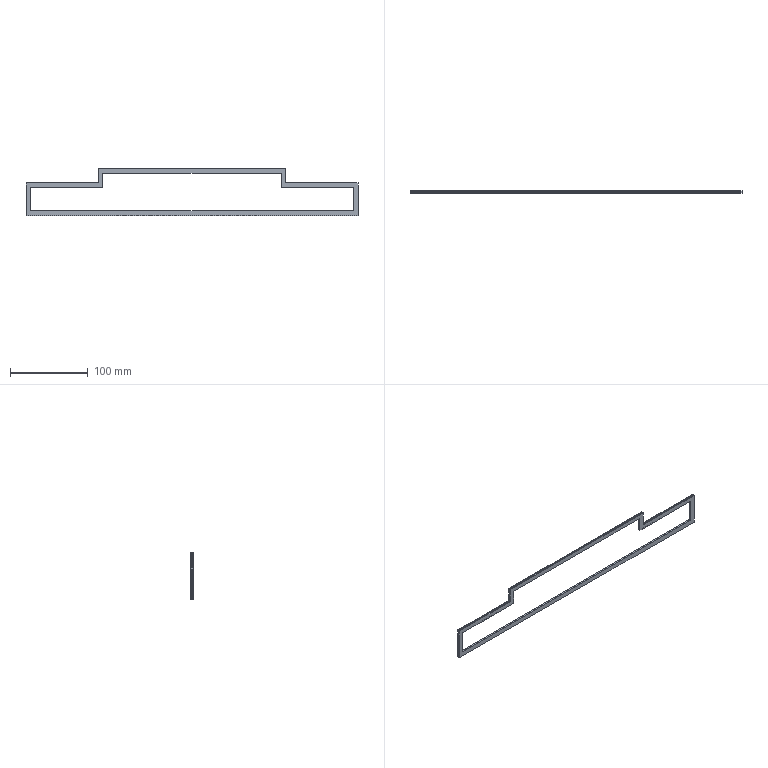Part | STEP file | _3000 | 1 solid | 36 faces | box 426.4 x 3 x 60.8 mm | volume 12335 mm3 | plane 36